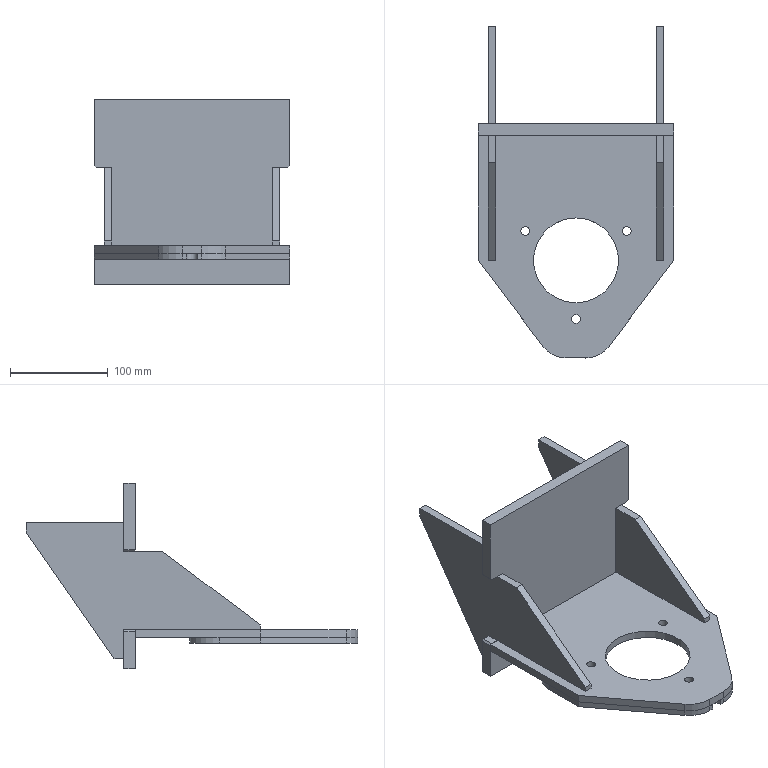Part | STEP file | HL4GZ-1.313.027 (front suspension bracket weldment) | 5 solids | 78 faces | box 200.001 x 340.001 x 190 mm | volume 984384 mm3 | plane 59 | cylinder 19 | commonest cylinder face diameters 60 x6 9 x3 12 x3 54 x3 604 x3 87 x1